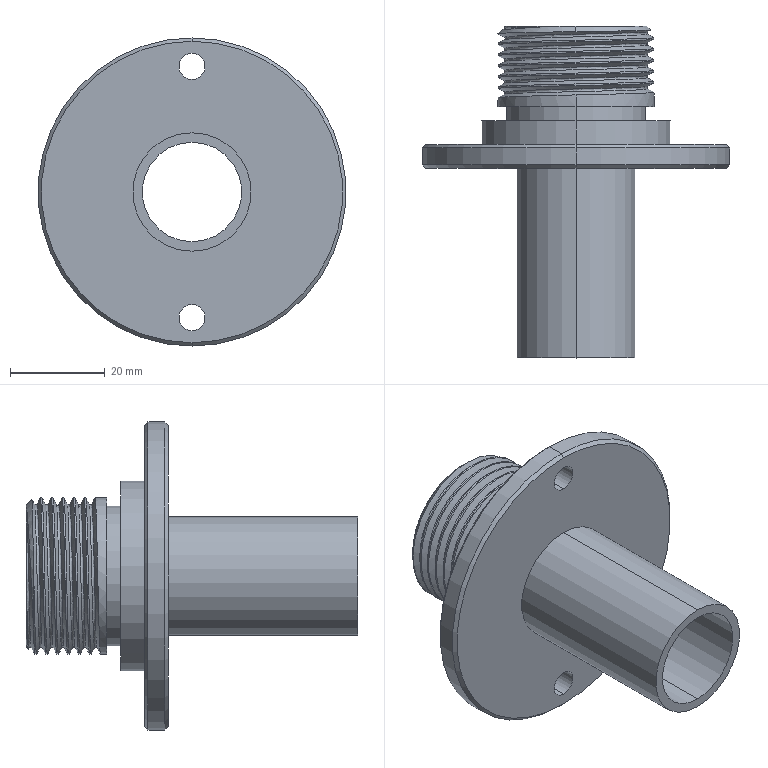Part | SolidWorks | features Helix 1, ICE 1, Revolution 1, SweepCut 1 | 1 solid | 44 faces | box 65 x 70 x 65 mm | volume 33296 mm3 | cylinder 27 | cone 7 | plane 7 | spline 3 | commonest cylinder face diameters 33 x13 5.5 x4 21 x2 25 x2 29.4 x2 40 x2